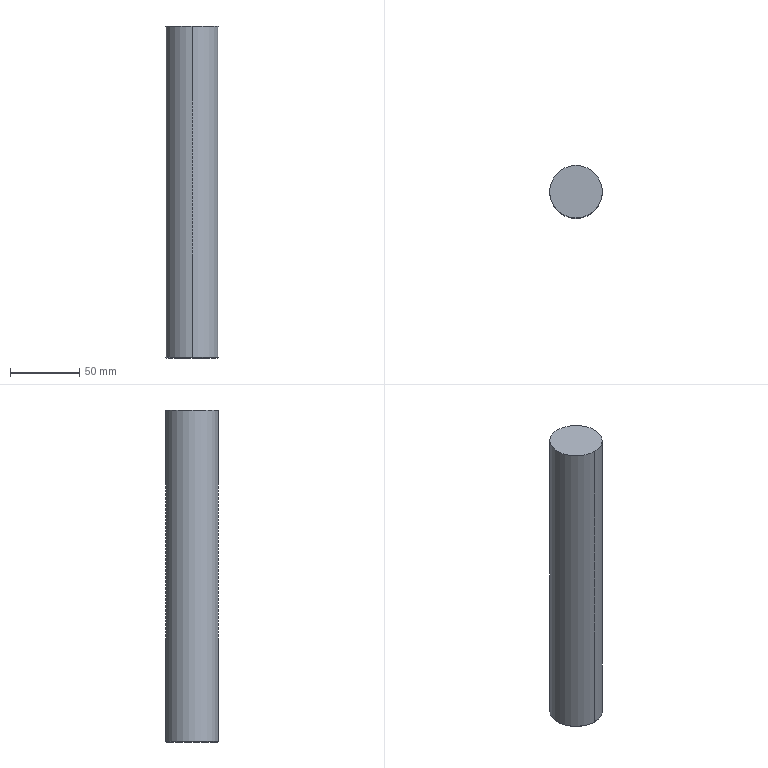Part | NX | features MYKP38-240_3 2 | 1 solid | 6 faces | box 38 x 38 x 240 mm | volume 272173 mm3 | cone 2 | plane 2 | cylinder 2 | commonest cylinder face diameters 38 x2
STEP:
#1=CARTESIAN_POINT('',(-420.023,300.595,-48.37));
#2=VERTEX_POINT('',#1);
#3=CARTESIAN_POINT('',(-420.023,300.095,-48.87));
#4=VERTEX_POINT('',#3);
#5=CARTESIAN_POINT('',(-420.023,300.095,-48.87));
#6=DIRECTION('',(0.000000003,0.7071,0.7071));
#7=VECTOR('',#6,1000.);
#8=LINE('',#5,#7);
#9=EDGE_CURVE('',#2,#4,#8,.F.);
#10=ORIENTED_EDGE('',*,*,#9,.F.);
#11=CARTESIAN_POINT('',(-420.023,262.595,-48.37));
#12=VERTEX_POINT('',#11);
#13=CARTESIAN_POINT('',(-420.023,281.595,-48.37));
#14=DIRECTION('',(0.,0.,-1.));
#15=DIRECTION('',(0.,1.,0.));
#16=AXIS2_PLACEMENT_3D('',#13,#14,#15);
#17=CIRCLE('',#16,19.);
#18=EDGE_CURVE('',#2,#12,#17,.T.);
#19=ORIENTED_EDGE('',*,*,#18,.T.);
#20=CARTESIAN_POINT('',(-420.023,263.095,-48.87));
#21=VERTEX_POINT('',#20);
#22=CARTESIAN_POINT('',(-420.023,263.095,-48.87));
#23=DIRECTION('',(-0.000000003,-0.7071,0.7071));
#24=VECTOR('',#23,1000.);
#25=LINE('',#22,#24);
#26=EDGE_CURVE('',#21,#12,#25,.T.);
#27=ORIENTED_EDGE('',*,*,#26,.F.);
#28=CARTESIAN_POINT('',(-420.023,281.595,-48.87));
#29=DIRECTION('',(0.,0.,-1.));
#30=DIRECTION('',(0.,1.,0.));
#31=AXIS2_PLACEMENT_3D('',#28,#29,#30);
#32=CIRCLE('',#31,18.5);
#33=EDGE_CURVE('',#4,#21,#32,.T.);
#34=ORIENTED_EDGE('',*,*,#33,.F.);
#35=EDGE_LOOP('',(#10,#19,#27,#34));
#36=FACE_BOUND('',#35,.T.);
#37=CARTESIAN_POINT('',(-420.023,281.595,-48.62));
#38=DIRECTION('',(0.,0.,1.));
#39=DIRECTION('',(1.,0.,0.));
#40=AXIS2_PLACEMENT_3D('',#37,#38,#39);
#41=CONICAL_SURFACE('',#40,18.75,0.7854);
#42=ADVANCED_FACE('',(#36),#41,.T.);
#43=ORIENTED_EDGE('',*,*,#26,.T.);
#44=CARTESIAN_POINT('',(-420.023,281.595,-48.37));
#45=DIRECTION('',(0.,0.,-1.));
#46=DIRECTION('',(0.,-1.,0.));
#47=AXIS2_PLACEMENT_3D('',#44,#45,#46);
#48=CIRCLE('',#47,19.);
#49=EDGE_CURVE('',#12,#2,#48,.T.);
#50=ORIENTED_EDGE('',*,*,#49,.T.);
#51=ORIENTED_EDGE('',*,*,#9,.T.);
#52=CARTESIAN_POINT('',(-420.023,281.595,-48.87));
#53=DIRECTION('',(0.,0.,-1.));
#54=DIRECTION('',(0.,-1.,0.));
#55=AXIS2_PLACEMENT_3D('',#52,#53,#54);
#56=CIRCLE('',#55,18.5);
#57=EDGE_CURVE('',#21,#4,#56,.T.);
#58=ORIENTED_EDGE('',*,*,#57,.F.);
#59=EDGE_LOOP('',(#43,#50,#51,#58));
#60=FACE_BOUND('',#59,.T.);
#61=CARTESIAN_POINT('',(-420.023,281.595,-48.62));
#62=DIRECTION('',(0.,0.,1.));
#63=DIRECTION('',(1.,0.,0.));
#64=AXIS2_PLACEMENT_3D('',#61,#62,#63);
#65=CONICAL_SURFACE('',#64,18.75,0.7854);
#66=ADVANCED_FACE('',(#60),#65,.T.);
#67=ORIENTED_EDGE('',*,*,#33,.T.);
#68=ORIENTED_EDGE('',*,*,#57,.T.);
#69=EDGE_LOOP('',(#67,#68));
#70=FACE_BOUND('',#69,.T.);
#71=CARTESIAN_POINT('',(-420.023,281.595,-48.87));
#72=DIRECTION('',(0.,0.,-1.));
#73=DIRECTION('',(0.,-1.,0.));
#74=AXIS2_PLACEMENT_3D('',#71,#72,#73);
#75=PLANE('',#74);
#76=ADVANCED_FACE('',(#70),#75,.T.);
#77=CARTESIAN_POINT('',(-420.023,300.595,138.13));
#78=VERTEX_POINT('',#77);
#79=CARTESIAN_POINT('',(-420.023,300.595,191.13));
#80=VERTEX_POINT('',#79);
#81=CARTESIAN_POINT('',(-420.023,300.595,61.63));
#82=DIRECTION('',(0.,0.000000019,1.));
#83=VECTOR('',#82,1000.);
#84=LINE('',#81,#83);
#85=EDGE_CURVE('',#78,#80,#84,.T.);
#86=ORIENTED_EDGE('',*,*,#85,.F.);
#87=CARTESIAN_POINT('',(-420.023,300.595,136.13));
#88=VERTEX_POINT('',#87);
#89=CARTESIAN_POINT('',(-420.023,300.595,61.63));
#90=DIRECTION('',(0.,0.000000019,1.));
#91=VECTOR('',#90,1000.);
#92=LINE('',#89,#91);
#93=EDGE_CURVE('',#88,#78,#92,.T.);
#94=ORIENTED_EDGE('',*,*,#93,.F.);
#95=CARTESIAN_POINT('',(-420.023,300.595,134.13));
#96=VERTEX_POINT('',#95);
#97=CARTESIAN_POINT('',(-420.023,300.595,59.63));
#98=DIRECTION('',(0.,0.000000019,1.));
#99=VECTOR('',#98,1000.);
#100=LINE('',#97,#99);
#101=EDGE_CURVE('',#96,#88,#100,.T.);
#102=ORIENTED_EDGE('',*,*,#101,.F.);
#103=CARTESIAN_POINT('',(-420.023,300.595,132.13));
#104=VERTEX_POINT('',#103);
#105=CARTESIAN_POINT('',(-420.023,300.595,57.63));
#106=DIRECTION('',(0.,0.000000019,1.));
#107=VECTOR('',#106,1000.);
#108=LINE('',#105,#107);
#109=EDGE_CURVE('',#104,#96,#108,.T.);
#110=ORIENTED_EDGE('',*,*,#109,.F.);
#111=CARTESIAN_POINT('',(-420.023,300.595,130.13));
#112=VERTEX_POINT('',#111);
#113=CARTESIAN_POINT('',(-420.023,300.595,55.63));
#114=DIRECTION('',(0.,0.000000019,1.));
#115=VECTOR('',#114,1000.);
#116=LINE('',#113,#115);
#117=EDGE_CURVE('',#112,#104,#116,.T.);
#118=ORIENTED_EDGE('',*,*,#117,.F.);
#119=CARTESIAN_POINT('',(-420.023,300.595,128.13));
#120=VERTEX_POINT('',#119);
#121=CARTESIAN_POINT('',(-420.023,300.595,53.63));
#122=DIRECTION('',(0.,0.000000019,1.));
#123=VECTOR('',#122,1000.);
#124=LINE('',#121,#123);
#125=EDGE_CURVE('',#120,#112,#124,.T.);
#126=ORIENTED_EDGE('',*,*,#125,.F.);
#127=CARTESIAN_POINT('',(-420.023,300.595,126.13));
#128=VERTEX_POINT('',#127);
#129=CARTESIAN_POINT('',(-420.023,300.595,51.63));
#130=DIRECTION('',(0.,0.000000019,1.));
#131=VECTOR('',#130,1000.);
#132=LINE('',#129,#131);
#133=EDGE_CURVE('',#128,#120,#132,.T.);
#134=ORIENTED_EDGE('',*,*,#133,.F.);
#135=CARTESIAN_POINT('',(-420.023,300.595,124.13));
#136=VERTEX_POINT('',#135);
#137=CARTESIAN_POINT('',(-420.023,300.595,49.63));
#138=DIRECTION('',(0.,0.000000019,1.));
#139=VECTOR('',#138,1000.);
#140=LINE('',#137,#139);
#141=EDGE_CURVE('',#136,#128,#140,.T.);
#142=ORIENTED_EDGE('',*,*,#141,.F.);
#143=CARTESIAN_POINT('',(-420.023,300.595,122.13));
#144=VERTEX_POINT('',#143);
#145=CARTESIAN_POINT('',(-420.023,300.595,47.63));
#146=DIRECTION('',(0.,0.000000019,1.));
#147=VECTOR('',#146,1000.);
#148=LINE('',#145,#147);
#149=EDGE_CURVE('',#144,#136,#148,.T.);
#150=ORIENTED_EDGE('',*,*,#149,.F.);
#151=CARTESIAN_POINT('',(-420.023,300.595,120.13));
#152=VERTEX_POINT('',#151);
#153=CARTESIAN_POINT('',(-420.023,300.595,45.63));
#154=DIRECTION('',(0.,0.000000019,1.));
#155=VECTOR('',#154,1000.);
#156=LINE('',#153,#155);
#157=EDGE_CURVE('',#152,#144,#156,.T.);
#158=ORIENTED_EDGE('',*,*,#157,.F.);
#159=CARTESIAN_POINT('',(-420.023,300.595,118.13));
#160=VERTEX_POINT('',#159);
#161=CARTESIAN_POINT('',(-420.023,300.595,43.63));
#162=DIRECTION('',(0.,0.000000019,1.));
#163=VECTOR('',#162,1000.);
#164=LINE('',#161,#163);
#165=EDGE_CURVE('',#160,#152,#164,.T.);
#166=ORIENTED_EDGE('',*,*,#165,.F.);
#167=CARTESIAN_POINT('',(-420.023,300.595,116.13));
#168=VERTEX_POINT('',#167);
#169=CARTESIAN_POINT('',(-420.023,300.595,41.63));
#170=DIRECTION('',(0.,0.000000019,1.));
#171=VECTOR('',#170,1000.);
#172=LINE('',#169,#171);
#173=EDGE_CURVE('',#168,#160,#172,.T.);
#174=ORIENTED_EDGE('',*,*,#173,.F.);
#175=CARTESIAN_POINT('',(-420.023,300.595,114.13));
#176=VERTEX_POINT('',#175);
#177=CARTESIAN_POINT('',(-420.023,300.595,39.63));
#178=DIRECTION('',(0.,0.000000019,1.));
#179=VECTOR('',#178,1000.);
#180=LINE('',#177,#179);
#181=EDGE_CURVE('',#176,#168,#180,.T.);
#182=ORIENTED_EDGE('',*,*,#181,.F.);
#183=CARTESIAN_POINT('',(-420.023,300.595,112.13));
#184=VERTEX_POINT('',#183);
#185=CARTESIAN_POINT('',(-420.023,300.595,37.63));
#186=DIRECTION('',(0.,0.000000019,1.));
#187=VECTOR('',#186,1000.);
#188=LINE('',#185,#187);
#189=EDGE_CURVE('',#184,#176,#188,.T.);
#190=ORIENTED_EDGE('',*,*,#189,.F.);
#191=CARTESIAN_POINT('',(-420.023,300.595,110.13));
#192=VERTEX_POINT('',#191);
#193=CARTESIAN_POINT('',(-420.023,300.595,35.63));
#194=DIRECTION('',(0.,0.000000019,1.));
#195=VECTOR('',#194,1000.);
#196=LINE('',#193,#195);
#197=EDGE_CURVE('',#192,#184,#196,.T.);
#198=ORIENTED_EDGE('',*,*,#197,.F.);
#199=CARTESIAN_POINT('',(-420.023,300.595,108.13));
#200=VERTEX_POINT('',#199);
#201=CARTESIAN_POINT('',(-420.023,300.595,33.63));
#202=DIRECTION('',(0.,0.000000019,1.));
#203=VECTOR('',#202,1000.);
#204=LINE('',#201,#203);
#205=EDGE_CURVE('',#200,#192,#204,.T.);
#206=ORIENTED_EDGE('',*,*,#205,.F.);
#207=CARTESIAN_POINT('',(-420.023,300.595,106.13));
#208=VERTEX_POINT('',#207);
#209=CARTESIAN_POINT('',(-420.023,300.595,31.63));
#210=DIRECTION('',(0.,0.000000019,1.));
#211=VECTOR('',#210,1000.);
#212=LINE('',#209,#211);
#213=EDGE_CURVE('',#208,#200,#212,.T.);
#214=ORIENTED_EDGE('',*,*,#213,.F.);
#215=CARTESIAN_POINT('',(-420.023,300.595,104.13));
#216=VERTEX_POINT('',#215);
#217=CARTESIAN_POINT('',(-420.023,300.595,29.63));
#218=DIRECTION('',(0.,0.000000019,1.));
#219=VECTOR('',#218,1000.);
#220=LINE('',#217,#219);
#221=EDGE_CURVE('',#216,#208,#220,.T.);
#222=ORIENTED_EDGE('',*,*,#221,.F.);
#223=CARTESIAN_POINT('',(-420.023,300.595,102.13));
#224=VERTEX_POINT('',#223);
#225=CARTESIAN_POINT('',(-420.023,300.595,27.63));
#226=DIRECTION('',(0.,0.000000019,1.));
#227=VECTOR('',#226,1000.);
#228=LINE('',#225,#227);
#229=EDGE_CURVE('',#224,#216,#228,.T.);
#230=ORIENTED_EDGE('',*,*,#229,.F.);
#231=CARTESIAN_POINT('',(-420.023,300.595,100.13));
#232=VERTEX_POINT('',#231);
#233=CARTESIAN_POINT('',(-420.023,300.595,25.63));
#234=DIRECTION('',(0.,0.000000019,1.));
#235=VECTOR('',#234,1000.);
#236=LINE('',#233,#235);
#237=EDGE_CURVE('',#232,#224,#236,.T.);
#238=ORIENTED_EDGE('',*,*,#237,.F.);
#239=CARTESIAN_POINT('',(-420.023,300.595,98.13));
#240=VERTEX_POINT('',#239);
#241=CARTESIAN_POINT('',(-420.023,300.595,23.63));
#242=DIRECTION('',(0.,0.000000019,1.));
#243=VECTOR('',#242,1000.);
#244=LINE('',#241,#243);
#245=EDGE_CURVE('',#240,#232,#244,.T.);
#246=ORIENTED_EDGE('',*,*,#245,.F.);
#247=CARTESIAN_POINT('',(-420.023,300.595,96.13));
#248=VERTEX_POINT('',#247);
#249=CARTESIAN_POINT('',(-420.023,300.595,21.63));
#250=DIRECTION('',(0.,0.000000019,1.));
#251=VECTOR('',#250,1000.);
#252=LINE('',#249,#251);
#253=EDGE_CURVE('',#248,#240,#252,.T.);
#254=ORIENTED_EDGE('',*,*,#253,.F.);
#255=CARTESIAN_POINT('',(-420.023,300.595,94.13));
#256=VERTEX_POINT('',#255);
#257=CARTESIAN_POINT('',(-420.023,300.595,19.63));
#258=DIRECTION('',(0.,0.000000019,1.));
#259=VECTOR('',#258,1000.);
#260=LINE('',#257,#259);
#261=EDGE_CURVE('',#256,#248,#260,.T.);
#262=ORIENTED_EDGE('',*,*,#261,.F.);
#263=CARTESIAN_POINT('',(-420.023,300.595,92.13));
#264=VERTEX_POINT('',#263);
#265=CARTESIAN_POINT('',(-420.023,300.595,17.63));
#266=DIRECTION('',(0.,0.000000019,1.));
#267=VECTOR('',#266,1000.);
#268=LINE('',#265,#267);
#269=EDGE_CURVE('',#264,#256,#268,.T.);
#270=ORIENTED_EDGE('',*,*,#269,.F.);
#271=CARTESIAN_POINT('',(-420.023,300.595,90.13));
#272=VERTEX_POINT('',#271);
#273=CARTESIAN_POINT('',(-420.023,300.595,15.63));
#274=DIRECTION('',(0.,0.000000019,1.));
#275=VECTOR('',#274,1000.);
#276=LINE('',#273,#275);
#277=EDGE_CURVE('',#272,#264,#276,.T.);
#278=ORIENTED_EDGE('',*,*,#277,.F.);
#279=CARTESIAN_POINT('',(-420.023,300.595,88.13));
#280=VERTEX_POINT('',#279);
#281=CARTESIAN_POINT('',(-420.023,300.595,13.63));
#282=DIRECTION('',(0.,0.000000019,1.));
#283=VECTOR('',#282,1000.);
#284=LINE('',#281,#283);
#285=EDGE_CURVE('',#280,#272,#284,.T.);
#286=ORIENTED_EDGE('',*,*,#285,.F.);
#287=CARTESIAN_POINT('',(-420.023,300.595,86.13));
#288=VERTEX_POINT('',#287);
#289=CARTESIAN_POINT('',(-420.023,300.595,11.63));
#290=DIRECTION('',(0.,0.000000019,1.));
#291=VECTOR('',#290,1000.);
#292=LINE('',#289,#291);
#293=EDGE_CURVE('',#288,#280,#292,.T.);
#294=ORIENTED_EDGE('',*,*,#293,.F.);
#295=CARTESIAN_POINT('',(-420.023,300.595,84.13));
#296=VERTEX_POINT('',#295);
#297=CARTESIAN_POINT('',(-420.023,300.595,9.63));
#298=DIRECTION('',(0.,0.000000019,1.));
#299=VECTOR('',#298,1000.);
#300=LINE('',#297,#299);
#301=EDGE_CURVE('',#296,#288,#300,.T.);
#302=ORIENTED_EDGE('',*,*,#301,.F.);
#303=CARTESIAN_POINT('',(-420.023,300.595,82.13));
#304=VERTEX_POINT('',#303);
#305=CARTESIAN_POINT('',(-420.023,300.595,7.63));
#306=DIRECTION('',(0.,0.000000019,1.));
#307=VECTOR('',#306,1000.);
#308=LINE('',#305,#307);
#309=EDGE_CURVE('',#304,#296,#308,.T.);
#310=ORIENTED_EDGE('',*,*,#309,.F.);
#311=CARTESIAN_POINT('',(-420.023,300.595,80.13));
#312=VERTEX_POINT('',#311);
#313=CARTESIAN_POINT('',(-420.023,300.595,5.63));
#314=DIRECTION('',(0.,0.000000019,1.));
#315=VECTOR('',#314,1000.);
#316=LINE('',#313,#315);
#317=EDGE_CURVE('',#312,#304,#316,.T.);
#318=ORIENTED_EDGE('',*,*,#317,.F.);
#319=CARTESIAN_POINT('',(-420.023,300.595,78.13));
#320=VERTEX_POINT('',#319);
#321=CARTESIAN_POINT('',(-420.023,300.595,3.63));
#322=DIRECTION('',(0.,0.000000019,1.));
#323=VECTOR('',#322,1000.);
#324=LINE('',#321,#323);
#325=EDGE_CURVE('',#320,#312,#324,.T.);
#326=ORIENTED_EDGE('',*,*,#325,.F.);
#327=CARTESIAN_POINT('',(-420.023,300.595,76.13));
#328=VERTEX_POINT('',#327);
#329=CARTESIAN_POINT('',(-420.023,300.595,1.63));
#330=DIRECTION('',(0.,0.000000019,1.));
#331=VECTOR('',#330,1000.);
#332=LINE('',#329,#331);
#333=EDGE_CURVE('',#328,#320,#332,.T.);
#334=ORIENTED_EDGE('',*,*,#333,.F.);
#335=CARTESIAN_POINT('',(-420.023,300.595,74.13));
#336=VERTEX_POINT('',#335);
#337=CARTESIAN_POINT('',(-420.023,300.595,-0.3701));
#338=DIRECTION('',(0.,0.000000019,1.));
#339=VECTOR('',#338,1000.);
#340=LINE('',#337,#339);
#341=EDGE_CURVE('',#336,#328,#340,.T.);
#342=ORIENTED_EDGE('',*,*,#341,.F.);
#343=CARTESIAN_POINT('',(-420.023,300.595,72.13));
#344=VERTEX_POINT('',#343);
#345=CARTESIAN_POINT('',(-420.023,300.595,-2.37));
#346=DIRECTION('',(0.,0.000000019,1.));
#347=VECTOR('',#346,1000.);
#348=LINE('',#345,#347);
#349=EDGE_CURVE('',#344,#336,#348,.T.);
#350=ORIENTED_EDGE('',*,*,#349,.F.);
#351=CARTESIAN_POINT('',(-420.023,300.595,70.13));
#352=VERTEX_POINT('',#351);
#353=CARTESIAN_POINT('',(-420.023,300.595,-4.37));
#354=DIRECTION('',(0.,0.000000019,1.));
#355=VECTOR('',#354,1000.);
#356=LINE('',#353,#355);
#357=EDGE_CURVE('',#352,#344,#356,.T.);
#358=ORIENTED_EDGE('',*,*,#357,.F.);
#359=CARTESIAN_POINT('',(-420.023,300.595,68.13));
#360=VERTEX_POINT('',#359);
#361=CARTESIAN_POINT('',(-420.023,300.595,-6.37));
#362=DIRECTION('',(0.,0.000000019,1.));
#363=VECTOR('',#362,1000.);
#364=LINE('',#361,#363);
#365=EDGE_CURVE('',#360,#352,#364,.T.);
#366=ORIENTED_EDGE('',*,*,#365,.F.);
#367=CARTESIAN_POINT('',(-420.023,300.595,66.13));
#368=VERTEX_POINT('',#367);
#369=CARTESIAN_POINT('',(-420.023,300.595,-8.37));
#370=DIRECTION('',(0.,0.000000019,1.));
#371=VECTOR('',#370,1000.);
#372=LINE('',#369,#371);
#373=EDGE_CURVE('',#368,#360,#372,.T.);
#374=ORIENTED_EDGE('',*,*,#373,.F.);
#375=CARTESIAN_POINT('',(-420.023,300.595,64.13));
#376=VERTEX_POINT('',#375);
#377=CARTESIAN_POINT('',(-420.023,300.595,-10.37));
#378=DIRECTION('',(0.,0.000000019,1.));
#379=VECTOR('',#378,1000.);
#380=LINE('',#377,#379);
#381=EDGE_CURVE('',#376,#368,#380,.T.);
#382=ORIENTED_EDGE('',*,*,#381,.F.);
#383=CARTESIAN_POINT('',(-420.023,300.595,62.13));
#384=VERTEX_POINT('',#383);
#385=CARTESIAN_POINT('',(-420.023,300.595,-12.37));
#386=DIRECTION('',(0.,0.000000019,1.));
#387=VECTOR('',#386,1000.);
#388=LINE('',#385,#387);
#389=EDGE_CURVE('',#384,#376,#388,.T.);
#390=ORIENTED_EDGE('',*,*,#389,.F.);
#391=CARTESIAN_POINT('',(-420.023,300.595,60.13));
#392=VERTEX_POINT('',#391);
#393=CARTESIAN_POINT('',(-420.023,300.595,-14.37));
#394=DIRECTION('',(0.,0.000000019,1.));
#395=VECTOR('',#394,1000.);
#396=LINE('',#393,#395);
#397=EDGE_CURVE('',#392,#384,#396,.T.);
#398=ORIENTED_EDGE('',*,*,#397,.F.);
#399=CARTESIAN_POINT('',(-420.023,300.595,58.13));
#400=VERTEX_POINT('',#399);
#401=CARTESIAN_POINT('',(-420.023,300.595,-16.37));
#402=DIRECTION('',(0.,0.000000019,1.));
#403=VECTOR('',#402,1000.);
#404=LINE('',#401,#403);
#405=EDGE_CURVE('',#400,#392,#404,.T.);
#406=ORIENTED_EDGE('',*,*,#405,.F.);
#407=CARTESIAN_POINT('',(-420.023,300.595,56.13));
#408=VERTEX_POINT('',#407);
#409=CARTESIAN_POINT('',(-420.023,300.595,-18.37));
#410=DIRECTION('',(0.,0.000000019,1.));
#411=VECTOR('',#410,1000.);
#412=LINE('',#409,#411);
#413=EDGE_CURVE('',#408,#400,#412,.T.);
#414=ORIENTED_EDGE('',*,*,#413,.F.);
#415=CARTESIAN_POINT('',(-420.023,300.595,54.13));
#416=VERTEX_POINT('',#415);
#417=CARTESIAN_POINT('',(-420.023,300.595,-20.37));
#418=DIRECTION('',(0.,0.000000019,1.));
#419=VECTOR('',#418,1000.);
#420=LINE('',#417,#419);
#421=EDGE_CURVE('',#416,#408,#420,.T.);
#422=ORIENTED_EDGE('',*,*,#421,.F.);
#423=CARTESIAN_POINT('',(-420.023,300.595,52.13));
#424=VERTEX_POINT('',#423);
#425=CARTESIAN_POINT('',(-420.023,300.595,-22.37));
#426=DIRECTION('',(0.,0.000000019,1.));
#427=VECTOR('',#426,1000.);
#428=LINE('',#425,#427);
#429=EDGE_CURVE('',#424,#416,#428,.T.);
#430=ORIENTED_EDGE('',*,*,#429,.F.);
#431=CARTESIAN_POINT('',(-420.023,300.595,50.13));
#432=VERTEX_POINT('',#431);
#433=CARTESIAN_POINT('',(-420.023,300.595,-24.37));
#434=DIRECTION('',(0.,0.000000019,1.));
#435=VECTOR('',#434,1000.);
#436=LINE('',#433,#435);
#437=EDGE_CURVE('',#432,#424,#436,.T.);
#438=ORIENTED_EDGE('',*,*,#437,.F.);
#439=CARTESIAN_POINT('',(-420.023,300.595,48.13));
#440=VERTEX_POINT('',#439);
#441=CARTESIAN_POINT('',(-420.023,300.595,-26.37));
#442=DIRECTION('',(0.,0.000000019,1.));
#443=VECTOR('',#442,1000.);
#444=LINE('',#441,#443);
#445=EDGE_CURVE('',#440,#432,#444,.T.);
#446=ORIENTED_EDGE('',*,*,#445,.F.);
#447=CARTESIAN_POINT('',(-420.023,300.595,46.13));
#448=VERTEX_POINT('',#447);
#449=CARTESIAN_POINT('',(-420.023,300.595,-28.37));
#450=DIRECTION('',(0.,0.000000019,1.));
#451=VECTOR('',#450,1000.);
#452=LINE('',#449,#451);
#453=EDGE_CURVE('',#448,#440,#452,.T.);
#454=ORIENTED_EDGE('',*,*,#453,.F.);
#455=CARTESIAN_POINT('',(-420.023,300.595,44.13));
#456=VERTEX_POINT('',#455);
#457=CARTESIAN_POINT('',(-420.023,300.595,-30.37));
#458=DIRECTION('',(0.,0.000000019,1.));
#459=VECTOR('',#458,1000.);
#460=LINE('',#457,#459);
#461=EDGE_CURVE('',#456,#448,#460,.T.);
#462=ORIENTED_EDGE('',*,*,#461,.F.);
#463=CARTESIAN_POINT('',(-420.023,300.595,42.13));
#464=VERTEX_POINT('',#463);
#465=CARTESIAN_POINT('',(-420.023,300.595,-32.37));
#466=DIRECTION('',(0.,0.000000019,1.));
#467=VECTOR('',#466,1000.);
#468=LINE('',#465,#467);
#469=EDGE_CURVE('',#464,#456,#468,.T.);
#470=ORIENTED_EDGE('',*,*,#469,.F.);
#471=CARTESIAN_POINT('',(-420.023,300.595,40.13));
#472=VERTEX_POINT('',#471);
#473=CARTESIAN_POINT('',(-420.023,300.595,-34.37));
#474=DIRECTION('',(0.,0.000000019,1.));
#475=VECTOR('',#474,1000.);
#476=LINE('',#473,#475);
#477=EDGE_CURVE('',#472,#464,#476,.T.);
#478=ORIENTED_EDGE('',*,*,#477,.F.);
#479=CARTESIAN_POINT('',(-420.023,300.595,38.13));
#480=VERTEX_POINT('',#479);
#481=CARTESIAN_POINT('',(-420.023,300.595,-36.37));
#482=DIRECTION('',(0.,0.000000019,1.));
#483=VECTOR('',#482,1000.);
#484=LINE('',#481,#483);
#485=EDGE_CURVE('',#480,#472,#484,.T.);
#486=ORIENTED_EDGE('',*,*,#485,.F.);
#487=CARTESIAN_POINT('',(-420.023,300.595,36.13));
#488=VERTEX_POINT('',#487);
#489=CARTESIAN_POINT('',(-420.023,300.595,-38.37));
#490=DIRECTION('',(0.,0.000000019,1.));
#491=VECTOR('',#490,1000.);
#492=LINE('',#489,#491);
#493=EDGE_CURVE('',#488,#480,#492,.T.);
#494=ORIENTED_EDGE('',*,*,#493,.F.);
#495=CARTESIAN_POINT('',(-420.023,300.595,34.13));
#496=VERTEX_POINT('',#495);
#497=CARTESIAN_POINT('',(-420.023,300.595,-40.37));
#498=DIRECTION('',(0.,0.000000019,1.));
#499=VECTOR('',#498,1000.);
#500=LINE('',#497,#499);
#501=EDGE_CURVE('',#496,#488,#500,.T.);
#502=ORIENTED_EDGE('',*,*,#501,.F.);
#503=CARTESIAN_POINT('',(-420.023,300.595,32.13));
#504=VERTEX_POINT('',#503);
#505=CARTESIAN_POINT('',(-420.023,300.595,-42.37));
#506=DIRECTION('',(0.,0.000000019,1.));
#507=VECTOR('',#506,1000.);
#508=LINE('',#505,#507);
#509=EDGE_CURVE('',#504,#496,#508,.T.);
#510=ORIENTED_EDGE('',*,*,#509,.F.);
#511=CARTESIAN_POINT('',(-420.023,300.595,30.13));
#512=VERTEX_POINT('',#511);
#513=CARTESIAN_POINT('',(-420.023,300.595,-44.37));
#514=DIRECTION('',(0.,0.000000019,1.));
#515=VECTOR('',#514,1000.);
#516=LINE('',#513,#515);
#517=EDGE_CURVE('',#512,#504,#516,.T.);
#518=ORIENTED_EDGE('',*,*,#517,.F.);
#519=CARTESIAN_POINT('',(-420.023,300.595,28.13));
#520=VERTEX_POINT('',#519);
#521=CARTESIAN_POINT('',(-420.023,300.595,-46.37));
#522=DIRECTION('',(0.,0.000000019,1.));
#523=VECTOR('',#522,1000.);
#524=LINE('',#521,#523);
#525=EDGE_CURVE('',#520,#512,#524,.T.);
#526=ORIENTED_EDGE('',*,*,#525,.F.);
#527=CARTESIAN_POINT('',(-420.023,300.595,26.13));
#528=VERTEX_POINT('',#527);
#529=CARTESIAN_POINT('',(-420.023,300.595,-48.37));
#530=DIRECTION('',(0.,0.000000019,1.));
#531=VECTOR('',#530,1000.);
#532=LINE('',#529,#531);
#533=EDGE_CURVE('',#528,#520,#532,.T.);
#534=ORIENTED_EDGE('',*,*,#533,.F.);
#535=CARTESIAN_POINT('',(-420.023,300.595,-48.37));
#536=DIRECTION('',(0.,0.000000019,1.));
#537=VECTOR('',#536,1000.);
#538=LINE('',#535,#537);
#539=EDGE_CURVE('',#2,#528,#538,.T.);
#540=ORIENTED_EDGE('',*,*,#539,.F.);
#541=ORIENTED_EDGE('',*,*,#49,.F.);
#542=CARTESIAN_POINT('',(-420.023,262.595,26.13));
#543=VERTEX_POINT('',#542);
#544=CARTESIAN_POINT('',(-420.023,262.595,-48.37));
#545=DIRECTION('',(0.,-0.000000019,1.));
#546=VECTOR('',#545,1000.);
#547=LINE('',#544,#546);
#548=EDGE_CURVE('',#543,#12,#547,.F.);
#549=ORIENTED_EDGE('',*,*,#548,.F.);
#550=CARTESIAN_POINT('',(-420.023,262.595,28.13));
#551=VERTEX_POINT('',#550);
#552=CARTESIAN_POINT('',(-420.023,262.595,-48.37));
#553=DIRECTION('',(0.,-0.000000019,1.));
#554=VECTOR('',#553,1000.);
#555=LINE('',#552,#554);
#556=EDGE_CURVE('',#551,#543,#555,.F.);
#557=ORIENTED_EDGE('',*,*,#556,.F.);
#558=CARTESIAN_POINT('',(-420.023,262.595,30.13));
#559=VERTEX_POINT('',#558);
#560=CARTESIAN_POINT('',(-420.023,262.595,-46.37));
#561=DIRECTION('',(0.,-0.000000019,1.));
#562=VECTOR('',#561,1000.);
#563=LINE('',#560,#562);
#564=EDGE_CURVE('',#559,#551,#563,.F.);
#565=ORIENTED_EDGE('',*,*,#564,.F.);
#566=CARTESIAN_POINT('',(-420.023,262.595,32.13));
#567=VERTEX_POINT('',#566);
#568=CARTESIAN_POINT('',(-420.023,262.595,-44.37));
#569=DIRECTION('',(0.,-0.000000019,1.));
#570=VECTOR('',#569,1000.);
#571=LINE('',#568,#570);
#572=EDGE_CURVE('',#567,#559,#571,.F.);
#573=ORIENTED_EDGE('',*,*,#572,.F.);
#574=CARTESIAN_POINT('',(-420.023,262.595,34.13));
#575=VERTEX_POINT('',#574);
#576=CARTESIAN_POINT('',(-420.023,262.595,-42.37));
#577=DIRECTION('',(0.,-0.000000019,1.));
#578=VECTOR('',#577,1000.);
#579=LINE('',#576,#578);
#580=EDGE_CURVE('',#575,#567,#579,.F.);
#581=ORIENTED_EDGE('',*,*,#580,.F.);
#582=CARTESIAN_POINT('',(-420.023,262.595,36.13));
#583=VERTEX_POINT('',#582);
#584=CARTESIAN_POINT('',(-420.023,262.595,-40.37));
#585=DIRECTION('',(0.,-0.000000019,1.));
#586=VECTOR('',#585,1000.);
#587=LINE('',#584,#586);
#588=EDGE_CURVE('',#583,#575,#587,.F.);
#589=ORIENTED_EDGE('',*,*,#588,.F.);
#590=CARTESIAN_POINT('',(-420.023,262.595,38.13));
#591=VERTEX_POINT('',#590);
#592=CARTESIAN_POINT('',(-420.023,262.595,-38.37));
#593=DIRECTION('',(0.,-0.000000019,1.));
#594=VECTOR('',#593,1000.);
#595=LINE('',#592,#594);
#596=EDGE_CURVE('',#591,#583,#595,.F.);
#597=ORIENTED_EDGE('',*,*,#596,.F.);
#598=CARTESIAN_POINT('',(-420.023,262.595,40.13));
#599=VERTEX_POINT('',#598);
#600=CARTESIAN_POINT('',(-420.023,262.595,-36.37));
#601=DIRECTION('',(0.,-0.000000019,1.));
#602=VECTOR('',#601,1000.);
#603=LINE('',#600,#602);
#604=EDGE_CURVE('',#599,#591,#603,.F.);
#605=ORIENTED_EDGE('',*,*,#604,.F.);
#606=CARTESIAN_POINT('',(-420.023,262.595,42.13));
#607=VERTEX_POINT('',#606);
#608=CARTESIAN_POINT('',(-420.023,262.595,-34.37));
#609=DIRECTION('',(0.,-0.000000019,1.));
#610=VECTOR('',#609,1000.);
#611=LINE('',#608,#610);
#612=EDGE_CURVE('',#607,#599,#611,.F.);
#613=ORIENTED_EDGE('',*,*,#612,.F.);
#614=CARTESIAN_POINT('',(-420.023,262.595,44.13));
#615=VERTEX_POINT('',#614);
#616=CARTESIAN_POINT('',(-420.023,262.595,-32.37));
#617=DIRECTION('',(0.,-0.000000019,1.));
#618=VECTOR('',#617,1000.);
#619=LINE('',#616,#618);
#620=EDGE_CURVE('',#615,#607,#619,.F.);
#621=ORIENTED_EDGE('',*,*,#620,.F.);
#622=CARTESIAN_POINT('',(-420.023,262.595,46.13));
#623=VERTEX_POINT('',#622);
#624=CARTESIAN_POINT('',(-420.023,262.595,-30.37));
#625=DIRECTION('',(0.,-0.000000019,1.));
#626=VECTOR('',#625,1000.);
#627=LINE('',#624,#626);
#628=EDGE_CURVE('',#623,#615,#627,.F.);
#629=ORIENTED_EDGE('',*,*,#628,.F.);
#630=CARTESIAN_POINT('',(-420.023,262.595,48.13));
#631=VERTEX_POINT('',#630);
#632=CARTESIAN_POINT('',(-420.023,262.595,-28.37));
#633=DIRECTION('',(0.,-0.000000019,1.));
#634=VECTOR('',#633,1000.);
#635=LINE('',#632,#634);
#636=EDGE_CURVE('',#631,#623,#635,.F.);
#637=ORIENTED_EDGE('',*,*,#636,.F.);
#638=CARTESIAN_POINT('',(-420.023,262.595,50.13));
#639=VERTEX_POINT('',#638);
#640=CARTESIAN_POINT('',(-420.023,262.595,-26.37));
#641=DIRECTION('',(0.,-0.000000019,1.));
#642=VECTOR('',#641,1000.);
#643=LINE('',#640,#642);
#644=EDGE_CURVE('',#639,#631,#643,.F.);
#645=ORIENTED_EDGE('',*,*,#644,.F.);
#646=CARTESIAN_POINT('',(-420.023,262.595,52.13));
#647=VERTEX_POINT('',#646);
#648=CARTESIAN_POINT('',(-420.023,262.595,-24.37));
#649=DIRECTION('',(0.,-0.000000019,1.));
#650=VECTOR('',#649,1000.);
#651=LINE('',#648,#650);
#652=EDGE_CURVE('',#647,#639,#651,.F.);
#653=ORIENTED_EDGE('',*,*,#652,.F.);
#654=CARTESIAN_POINT('',(-420.023,262.595,54.13));
#655=VERTEX_POINT('',#654);
#656=CARTESIAN_POINT('',(-420.023,262.595,-22.37));
#657=DIRECTION('',(0.,-0.000000019,1.));
#658=VECTOR('',#657,1000.);
#659=LINE('',#656,#658);
#660=EDGE_CURVE('',#655,#647,#659,.F.);
#661=ORIENTED_EDGE('',*,*,#660,.F.);
#662=CARTESIAN_POINT('',(-420.023,262.595,56.13));
#663=VERTEX_POINT('',#662);
#664=CARTESIAN_POINT('',(-420.023,262.595,-20.37));
#665=DIRECTION('',(0.,-0.000000019,1.));
#666=VECTOR('',#665,1000.);
#667=LINE('',#664,#666);
#668=EDGE_CURVE('',#663,#655,#667,.F.);
#669=ORIENTED_EDGE('',*,*,#668,.F.);
#670=CARTESIAN_POINT('',(-420.023,262.595,58.13));
#671=VERTEX_POINT('',#670);
#672=CARTESIAN_POINT('',(-420.023,262.595,-18.37));
#673=DIRECTION('',(0.,-0.000000019,1.));
#674=VECTOR('',#673,1000.);
#675=LINE('',#672,#674);
#676=EDGE_CURVE('',#671,#663,#675,.F.);
#677=ORIENTED_EDGE('',*,*,#676,.F.);
#678=CARTESIAN_POINT('',(-420.023,262.595,60.13));
#679=VERTEX_POINT('',#678);
#680=CARTESIAN_POINT('',(-420.023,262.595,-16.37));
#681=DIRECTION('',(0.,-0.000000019,1.));
#682=VECTOR('',#681,1000.);
#683=LINE('',#680,#682);
#684=EDGE_CURVE('',#679,#671,#683,.F.);
#685=ORIENTED_EDGE('',*,*,#684,.F.);
#686=CARTESIAN_POINT('',(-420.023,262.595,62.13));
#687=VERTEX_POINT('',#686);
#688=CARTESIAN_POINT('',(-420.023,262.595,-14.37));
#689=DIRECTION('',(0.,-0.000000019,1.));
#690=VECTOR('',#689,1000.);
#691=LINE('',#688,#690);
#692=EDGE_CURVE('',#687,#679,#691,.F.);
#693=ORIENTED_EDGE('',*,*,#692,.F.);
#694=CARTESIAN_POINT('',(-420.023,262.595,64.13));
#695=VERTEX_POINT('',#694);
#696=CARTESIAN_POINT('',(-420.023,262.595,-12.37));
#697=DIRECTION('',(0.,-0.000000019,1.));
#698=VECTOR('',#697,1000.);
#699=LINE('',#696,#698);
#700=EDGE_CURVE('',#695,#687,#699,.F.);
#701=ORIENTED_EDGE('',*,*,#700,.F.);
#702=CARTESIAN_POINT('',(-420.023,262.595,66.13));
#703=VERTEX_POINT('',#702);
#704=CARTESIAN_POINT('',(-420.023,262.595,-10.37));
#705=DIRECTION('',(0.,-0.000000019,1.));
#706=VECTOR('',#705,1000.);
#707=LINE('',#704,#706);
#708=EDGE_CURVE('',#703,#695,#707,.F.);
#709=ORIENTED_EDGE('',*,*,#708,.F.);
#710=CARTESIAN_POINT('',(-420.023,262.595,68.13));
#711=VERTEX_POINT('',#710);
#712=CARTESIAN_POINT('',(-420.023,262.595,-8.37));
#713=DIRECTION('',(0.,-0.000000019,1.));
#714=VECTOR('',#713,1000.);
#715=LINE('',#712,#714);
#716=EDGE_CURVE('',#711,#703,#715,.F.);
#717=ORIENTED_EDGE('',*,*,#716,.F.);
#718=CARTESIAN_POINT('',(-420.023,262.595,70.13));
#719=VERTEX_POINT('',#718);
#720=CARTESIAN_POINT('',(-420.023,262.595,-6.37));
#721=DIRECTION('',(0.,-0.000000019,1.));
#722=VECTOR('',#721,1000.);
#723=LINE('',#720,#722);
#724=EDGE_CURVE('',#719,#711,#723,.F.);
#725=ORIENTED_EDGE('',*,*,#724,.F.);
#726=CARTESIAN_POINT('',(-420.023,262.595,72.13));
#727=VERTEX_POINT('',#726);
#728=CARTESIAN_POINT('',(-420.023,262.595,-4.37));
#729=DIRECTION('',(0.,-0.000000019,1.));
#730=VECTOR('',#729,1000.);
#731=LINE('',#728,#730);
#732=EDGE_CURVE('',#727,#719,#731,.F.);
#733=ORIENTED_EDGE('',*,*,#732,.F.);
#734=CARTESIAN_POINT('',(-420.023,262.595,74.13));
#735=VERTEX_POINT('',#734);
#736=CARTESIAN_POINT('',(-420.023,262.595,-2.37));
#737=DIRECTION('',(0.,-0.000000019,1.));
#738=VECTOR('',#737,1000.);
#739=LINE('',#736,#738);
#740=EDGE_CURVE('',#735,#727,#739,.F.);
#741=ORIENTED_EDGE('',*,*,#740,.F.);
#742=CARTESIAN_POINT('',(-420.023,262.595,76.13));
#743=VERTEX_POINT('',#742);
#744=CARTESIAN_POINT('',(-420.023,262.595,-0.3701));
#745=DIRECTION('',(0.,-0.000000019,1.));
#746=VECTOR('',#745,1000.);
#747=LINE('',#744,#746);
#748=EDGE_CURVE('',#743,#735,#747,.F.);
#749=ORIENTED_EDGE('',*,*,#748,.F.);
#750=CARTESIAN_POINT('',(-420.023,262.595,78.13));
#751=VERTEX_POINT('',#750);
#752=CARTESIAN_POINT('',(-420.023,262.595,1.63));
#753=DIRECTION('',(0.,-0.000000019,1.));
#754=VECTOR('',#753,1000.);
#755=LINE('',#752,#754);
#756=EDGE_CURVE('',#751,#743,#755,.F.);
#757=ORIENTED_EDGE('',*,*,#756,.F.);
#758=CARTESIAN_POINT('',(-420.023,262.595,80.13));
#759=VERTEX_POINT('',#758);
#760=CARTESIAN_POINT('',(-420.023,262.595,3.63));
#761=DIRECTION('',(0.,-0.000000019,1.));
#762=VECTOR('',#761,1000.);
#763=LINE('',#760,#762);
#764=EDGE_CURVE('',#759,#751,#763,.F.);
#765=ORIENTED_EDGE('',*,*,#764,.F.);
#766=CARTESIAN_POINT('',(-420.023,262.595,82.13));
#767=VERTEX_POINT('',#766);
#768=CARTESIAN_POINT('',(-420.023,262.595,5.63));
#769=DIRECTION('',(0.,-0.000000019,1.));
#770=VECTOR('',#769,1000.);
#771=LINE('',#768,#770);
#772=EDGE_CURVE('',#767,#759,#771,.F.);
#773=ORIENTED_EDGE('',*,*,#772,.F.);
#774=CARTESIAN_POINT('',(-420.023,262.595,84.13));
#775=VERTEX_POINT('',#774);
#776=CARTESIAN_POINT('',(-420.023,262.595,7.63));
#777=DIRECTION('',(0.,-0.000000019,1.));
#778=VECTOR('',#777,1000.);
#779=LINE('',#776,#778);
#780=EDGE_CURVE('',#775,#767,#779,.F.);
#781=ORIENTED_EDGE('',*,*,#780,.F.);
#782=CARTESIAN_POINT('',(-420.023,262.595,86.13));
#783=VERTEX_POINT('',#782);
#784=CARTESIAN_POINT('',(-420.023,262.595,9.63));
#785=DIRECTION('',(0.,-0.000000019,1.));
#786=VECTOR('',#785,1000.);
#787=LINE('',#784,#786);
#788=EDGE_CURVE('',#783,#775,#787,.F.);
#789=ORIENTED_EDGE('',*,*,#788,.F.);
#790=CARTESIAN_POINT('',(-420.023,262.595,88.13));
#791=VERTEX_POINT('',#790);
#792=CARTESIAN_POINT('',(-420.023,262.595,11.63));
#793=DIRECTION('',(0.,-0.000000019,1.));
#794=VECTOR('',#793,1000.);
#795=LINE('',#792,#794);
#796=EDGE_CURVE('',#791,#783,#795,.F.);
#797=ORIENTED_EDGE('',*,*,#796,.F.);
#798=CARTESIAN_POINT('',(-420.023,262.595,90.13));
#799=VERTEX_POINT('',#798);
#800=CARTESIAN_POINT('',(-420.023,262.595,13.63));
#801=DIRECTION('',(0.,-0.000000019,1.));
#802=VECTOR('',#801,1000.);
#803=LINE('',#800,#802);
#804=EDGE_CURVE('',#799,#791,#803,.F.);
#805=ORIENTED_EDGE('',*,*,#804,.F.);
#806=CARTESIAN_POINT('',(-420.023,262.595,92.13));
#807=VERTEX_POINT('',#806);
#808=CARTESIAN_POINT('',(-420.023,262.595,15.63));
#809=DIRECTION('',(0.,-0.000000019,1.));
#810=VECTOR('',#809,1000.);
#811=LINE('',#808,#810);
#812=EDGE_CURVE('',#807,#799,#811,.F.);
#813=ORIENTED_EDGE('',*,*,#812,.F.);
#814=CARTESIAN_POINT('',(-420.023,262.595,94.13));
#815=VERTEX_POINT('',#814);
#816=CARTESIAN_POINT('',(-420.023,262.595,17.63));
#817=DIRECTION('',(0.,-0.000000019,1.));
#818=VECTOR('',#817,1000.);
#819=LINE('',#816,#818);
#820=EDGE_CURVE('',#815,#807,#819,.F.);
#821=ORIENTED_EDGE('',*,*,#820,.F.);
#822=CARTESIAN_POINT('',(-420.023,262.595,96.13));
#823=VERTEX_POINT('',#822);
#824=CARTESIAN_POINT('',(-420.023,262.595,19.63));
#825=DIRECTION('',(0.,-0.000000019,1.));
#826=VECTOR('',#825,1000.);
#827=LINE('',#824,#826);
#828=EDGE_CURVE('',#823,#815,#827,.F.);
#829=ORIENTED_EDGE('',*,*,#828,.F.);
#830=CARTESIAN_POINT('',(-420.023,262.595,98.13));
#831=VERTEX_POINT('',#830);
#832=CARTESIAN_POINT('',(-420.023,262.595,21.63));
#833=DIRECTION('',(0.,-0.000000019,1.));
#834=VECTOR('',#833,1000.);
#835=LINE('',#832,#834);
#836=EDGE_CURVE('',#831,#823,#835,.F.);
#837=ORIENTED_EDGE('',*,*,#836,.F.);
#838=CARTESIAN_POINT('',(-420.023,262.595,100.13));
#839=VERTEX_POINT('',#838);
#840=CARTESIAN_POINT('',(-420.023,262.595,23.63));
#841=DIRECTION('',(0.,-0.000000019,1.));
#842=VECTOR('',#841,1000.);
#843=LINE('',#840,#842);
#844=EDGE_CURVE('',#839,#831,#843,.F.);
#845=ORIENTED_EDGE('',*,*,#844,.F.);
#846=CARTESIAN_POINT('',(-420.023,262.595,102.13));
#847=VERTEX_POINT('',#846);
#848=CARTESIAN_POINT('',(-420.023,262.595,25.63));
#849=DIRECTION('',(0.,-0.000000019,1.));
#850=VECTOR('',#849,1000.);
#851=LINE('',#848,#850);
#852=EDGE_CURVE('',#847,#839,#851,.F.);
#853=ORIENTED_EDGE('',*,*,#852,.F.);
#854=CARTESIAN_POINT('',(-420.023,262.595,104.13));
#855=VERTEX_POINT('',#854);
#856=CARTESIAN_POINT('',(-420.023,262.595,27.63));
#857=DIRECTION('',(0.,-0.000000019,1.));
#858=VECTOR('',#857,1000.);
#859=LINE('',#856,#858);
#860=EDGE_CURVE('',#855,#847,#859,.F.);
#861=ORIENTED_EDGE('',*,*,#860,.F.);
#862=CARTESIAN_POINT('',(-420.023,262.595,106.13));
#863=VERTEX_POINT('',#862);
#864=CARTESIAN_POINT('',(-420.023,262.595,29.63));
#865=DIRECTION('',(0.,-0.000000019,1.));
#866=VECTOR('',#865,1000.);
#867=LINE('',#864,#866);
#868=EDGE_CURVE('',#863,#855,#867,.F.);
#869=ORIENTED_EDGE('',*,*,#868,.F.);
#870=CARTESIAN_POINT('',(-420.023,262.595,108.13));
#871=VERTEX_POINT('',#870);
#872=CARTESIAN_POINT('',(-420.023,262.595,31.63));
#873=DIRECTION('',(0.,-0.000000019,1.));
#874=VECTOR('',#873,1000.);
#875=LINE('',#872,#874);
#876=EDGE_CURVE('',#871,#863,#875,.F.);
#877=ORIENTED_EDGE('',*,*,#876,.F.);
#878=CARTESIAN_POINT('',(-420.023,262.595,110.13));
#879=VERTEX_POINT('',#878);
#880=CARTESIAN_POINT('',(-420.023,262.595,33.63));
#881=DIRECTION('',(0.,-0.000000019,1.));
#882=VECTOR('',#881,1000.);
#883=LINE('',#880,#882);
#884=EDGE_CURVE('',#879,#871,#883,.F.);
#885=ORIENTED_EDGE('',*,*,#884,.F.);
#886=CARTESIAN_POINT('',(-420.023,262.595,112.13));
#887=VERTEX_POINT('',#886);
#888=CARTESIAN_POINT('',(-420.023,262.595,35.63));
#889=DIRECTION('',(0.,-0.000000019,1.));
#890=VECTOR('',#889,1000.);
#891=LINE('',#888,#890);
#892=EDGE_CURVE('',#887,#879,#891,.F.);
#893=ORIENTED_EDGE('',*,*,#892,.F.);
#894=CARTESIAN_POINT('',(-420.023,262.595,114.13));
#895=VERTEX_POINT('',#894);
#896=CARTESIAN_POINT('',(-420.023,262.595,37.63));
#897=DIRECTION('',(0.,-0.000000019,1.));
#898=VECTOR('',#897,1000.);
#899=LINE('',#896,#898);
#900=EDGE_CURVE('',#895,#887,#899,.F.);
#901=ORIENTED_EDGE('',*,*,#900,.F.);
#902=CARTESIAN_POINT('',(-420.023,262.595,116.13));
#903=VERTEX_POINT('',#902);
#904=CARTESIAN_POINT('',(-420.023,262.595,39.63));
#905=DIRECTION('',(0.,-0.000000019,1.));
#906=VECTOR('',#905,1000.);
#907=LINE('',#904,#906);
#908=EDGE_CURVE('',#903,#895,#907,.F.);
#909=ORIENTED_EDGE('',*,*,#908,.F.);
#910=CARTESIAN_POINT('',(-420.023,262.595,118.13));
#911=VERTEX_POINT('',#910);
#912=CARTESIAN_POINT('',(-420.023,262.595,41.63));
#913=DIRECTION('',(0.,-0.000000019,1.));
#914=VECTOR('',#913,1000.);
#915=LINE('',#912,#914);
#916=EDGE_CURVE('',#911,#903,#915,.F.);
#917=ORIENTED_EDGE('',*,*,#916,.F.);
#918=CARTESIAN_POINT('',(-420.023,262.595,120.13));
#919=VERTEX_POINT('',#918);
#920=CARTESIAN_POINT('',(-420.023,262.595,43.63));
#921=DIRECTION('',(0.,-0.000000019,1.));
#922=VECTOR('',#921,1000.);
#923=LINE('',#920,#922);
#924=EDGE_CURVE('',#919,#911,#923,.F.);
#925=ORIENTED_EDGE('',*,*,#924,.F.);
#926=CARTESIAN_POINT('',(-420.023,262.595,122.13));
#927=VERTEX_POINT('',#926);
#928=CARTESIAN_POINT('',(-420.023,262.595,45.63));
#929=DIRECTION('',(0.,-0.000000019,1.));
#930=VECTOR('',#929,1000.);
#931=LINE('',#928,#930);
#932=EDGE_CURVE('',#927,#919,#931,.F.);
#933=ORIENTED_EDGE('',*,*,#932,.F.);
#934=CARTESIAN_POINT('',(-420.023,262.595,124.13));
#935=VERTEX_POINT('',#934);
#936=CARTESIAN_POINT('',(-420.023,262.595,47.63));
#937=DIRECTION('',(0.,-0.000000019,1.));
#938=VECTOR('',#937,1000.);
#939=LINE('',#936,#938);
#940=EDGE_CURVE('',#935,#927,#939,.F.);
#941=ORIENTED_EDGE('',*,*,#940,.F.);
#942=CARTESIAN_POINT('',(-420.023,262.595,126.13));
#943=VERTEX_POINT('',#942);
#944=CARTESIAN_POINT('',(-420.023,262.595,49.63));
#945=DIRECTION('',(0.,-0.000000019,1.));
#946=VECTOR('',#945,1000.);
#947=LINE('',#944,#946);
#948=EDGE_CURVE('',#943,#935,#947,.F.);
#949=ORIENTED_EDGE('',*,*,#948,.F.);
#950=CARTESIAN_POINT('',(-420.023,262.595,128.13));
#951=VERTEX_POINT('',#950);
#952=CARTESIAN_POINT('',(-420.023,262.595,51.63));
#953=DIRECTION('',(0.,-0.000000019,1.));
#954=VECTOR('',#953,1000.);
#955=LINE('',#952,#954);
#956=EDGE_CURVE('',#951,#943,#955,.F.);
#957=ORIENTED_EDGE('',*,*,#956,.F.);
#958=CARTESIAN_POINT('',(-420.023,262.595,130.13));
#959=VERTEX_POINT('',#958);
#960=CARTESIAN_POINT('',(-420.023,262.595,53.63));
#961=DIRECTION('',(0.,-0.000000019,1.));
#962=VECTOR('',#961,1000.);
#963=LINE('',#960,#962);
#964=EDGE_CURVE('',#959,#951,#963,.F.);
#965=ORIENTED_EDGE('',*,*,#964,.F.);
#966=CARTESIAN_POINT('',(-420.023,262.595,132.13));
#967=VERTEX_POINT('',#966);
#968=CARTESIAN_POINT('',(-420.023,262.595,55.63));
#969=DIRECTION('',(0.,-0.000000019,1.));
#970=VECTOR('',#969,1000.);
#971=LINE('',#968,#970);
#972=EDGE_CURVE('',#967,#959,#971,.F.);
#973=ORIENTED_EDGE('',*,*,#972,.F.);
#974=CARTESIAN_POINT('',(-420.023,262.595,134.13));
#975=VERTEX_POINT('',#974);
#976=CARTESIAN_POINT('',(-420.023,262.595,57.63));
#977=DIRECTION('',(0.,-0.000000019,1.));
#978=VECTOR('',#977,1000.);
#979=LINE('',#976,#978);
#980=EDGE_CURVE('',#975,#967,#979,.F.);
#981=ORIENTED_EDGE('',*,*,#980,.F.);
#982=CARTESIAN_POINT('',(-420.023,262.595,136.13));
#983=VERTEX_POINT('',#982);
#984=CARTESIAN_POINT('',(-420.023,262.595,59.63));
#985=DIRECTION('',(0.,-0.000000019,1.));
#986=VECTOR('',#985,1000.);
#987=LINE('',#984,#986);
#988=EDGE_CURVE('',#983,#975,#987,.F.);
#989=ORIENTED_EDGE('',*,*,#988,.F.);
#990=CARTESIAN_POINT('',(-420.023,262.595,138.13));
#991=VERTEX_POINT('',#990);
#992=CARTESIAN_POINT('',(-420.023,262.595,61.63));
#993=DIRECTION('',(0.,-0.000000019,1.));
#994=VECTOR('',#993,1000.);
#995=LINE('',#992,#994);
#996=EDGE_CURVE('',#991,#983,#995,.F.);
#997=ORIENTED_EDGE('',*,*,#996,.F.);
#998=CARTESIAN_POINT('',(-420.023,262.595,191.13));
#999=VERTEX_POINT('',#998);
#1000=CARTESIAN_POINT('',(-420.023,262.595,61.63));
#1001=DIRECTION('',(0.,-0.000000019,1.));
#1002=VECTOR('',#1001,1000.);
#1003=LINE('',#1000,#1002);
#1004=EDGE_CURVE('',#999,#991,#1003,.F.);
#1005=ORIENTED_EDGE('',*,*,#1004,.F.);
#1006=CARTESIAN_POINT('',(-420.023,281.595,191.13));
#1007=DIRECTION('',(0.,0.,1.));
#1008=DIRECTION('',(0.,1.,0.));
#1009=AXIS2_PLACEMENT_3D('',#1006,#1007,#1008);
#1010=CIRCLE('',#1009,19.);
#1011=EDGE_CURVE('',#80,#999,#1010,.T.);
#1012=ORIENTED_EDGE('',*,*,#1011,.F.);
#1013=EDGE_LOOP('',(#86,#94,#102,#110,#118,#126,#134,#142,#150,#158,#166,#174,#182,#190,#198,#206,#214,#222,#230,#238,#246,#254,#262,#270,#278,#286,#294,#302,#310,#318,#326,#334,#342,#350,#358,#366,#374,#382,#390,#398,#406,#414,#422,#430,#438,#446,#454,#462,#470,#478,#486,#494,#502,#510,#518,#526,#534,#540,#541,#549,#557,#565,#573,#581,#589,#597,#605,#613,#621,#629,#637,#645,#653,#661,#669,#677,#685,#693,#701,#709,#717,#725,#733,#741,#749,#757,#765,#773,#781,#789,#797,#805,#813,#821,#829,#837,#845,#853,#861,#869,#877,#885,#893,#901,#909,#917,#925,#933,#941,#949,#957,#965,#973,#981,#989,#997,#1005,#1012));
#1014=FACE_BOUND('',#1013,.T.);
#1015=CARTESIAN_POINT('',(-420.023,281.595,61.13));
#1016=DIRECTION('',(0.,0.,-1.));
#1017=DIRECTION('',(0.,1.,0.));
#1018=AXIS2_PLACEMENT_3D('',#1015,#1016,#1017);
#1019=CYLINDRICAL_SURFACE('',#1018,19.);
#1020=ADVANCED_FACE('',(#1014),#1019,.T.);
#1021=ORIENTED_EDGE('',*,*,#1011,.T.);
#1022=CARTESIAN_POINT('',(-420.023,281.595,191.13));
#1023=DIRECTION('',(0.,0.,1.));
#1024=DIRECTION('',(0.,-1.,0.));
#1025=AXIS2_PLACEMENT_3D('',#1022,#1023,#1024);
#1026=CIRCLE('',#1025,19.);
#1027=EDGE_CURVE('',#999,#80,#1026,.T.);
#1028=ORIENTED_EDGE('',*,*,#1027,.T.);
#1029=EDGE_LOOP('',(#1021,#1028));
#1030=FACE_BOUND('',#1029,.T.);
#1031=CARTESIAN_POINT('',(-382.523,219.595,191.13));
#1032=DIRECTION('',(0.,0.,1.));
#1033=DIRECTION('',(1.,0.,0.));
#1034=AXIS2_PLACEMENT_3D('',#1031,#1032,#1033);
#1035=PLANE('',#1034);
#1036=ADVANCED_FACE('',(#1030),#1035,.T.);
#1037=ORIENTED_EDGE('',*,*,#1004,.T.);
#1038=ORIENTED_EDGE('',*,*,#996,.T.);
#1039=ORIENTED_EDGE('',*,*,#988,.T.);
#1040=ORIENTED_EDGE('',*,*,#980,.T.);
#1041=ORIENTED_EDGE('',*,*,#972,.T.);
#1042=ORIENTED_EDGE('',*,*,#964,.T.);
#1043=ORIENTED_EDGE('',*,*,#956,.T.);
#1044=ORIENTED_EDGE('',*,*,#948,.T.);
#1045=ORIENTED_EDGE('',*,*,#940,.T.);
#1046=ORIENTED_EDGE('',*,*,#932,.T.);
#1047=ORIENTED_EDGE('',*,*,#924,.T.);
#1048=ORIENTED_EDGE('',*,*,#916,.T.);
#1049=ORIENTED_EDGE('',*,*,#908,.T.);
#1050=ORIENTED_EDGE('',*,*,#900,.T.);
#1051=ORIENTED_EDGE('',*,*,#892,.T.);
#1052=ORIENTED_EDGE('',*,*,#884,.T.);
#1053=ORIENTED_EDGE('',*,*,#876,.T.);
#1054=ORIENTED_EDGE('',*,*,#868,.T.);
#1055=ORIENTED_EDGE('',*,*,#860,.T.);
#1056=ORIENTED_EDGE('',*,*,#852,.T.);
#1057=ORIENTED_EDGE('',*,*,#844,.T.);
#1058=ORIENTED_EDGE('',*,*,#836,.T.);
#1059=ORIENTED_EDGE('',*,*,#828,.T.);
#1060=ORIENTED_EDGE('',*,*,#820,.T.);
#1061=ORIENTED_EDGE('',*,*,#812,.T.);
#1062=ORIENTED_EDGE('',*,*,#804,.T.);
#1063=ORIENTED_EDGE('',*,*,#796,.T.);
#1064=ORIENTED_EDGE('',*,*,#788,.T.);
#1065=ORIENTED_EDGE('',*,*,#780,.T.);
#1066=ORIENTED_EDGE('',*,*,#772,.T.);
#1067=ORIENTED_EDGE('',*,*,#764,.T.);
#1068=ORIENTED_EDGE('',*,*,#756,.T.);
#1069=ORIENTED_EDGE('',*,*,#748,.T.);
#1070=ORIENTED_EDGE('',*,*,#740,.T.);
#1071=ORIENTED_EDGE('',*,*,#732,.T.);
#1072=ORIENTED_EDGE('',*,*,#724,.T.);
#1073=ORIENTED_EDGE('',*,*,#716,.T.);
#1074=ORIENTED_EDGE('',*,*,#708,.T.);
#1075=ORIENTED_EDGE('',*,*,#700,.T.);
#1076=ORIENTED_EDGE('',*,*,#692,.T.);
#1077=ORIENTED_EDGE('',*,*,#684,.T.);
#1078=ORIENTED_EDGE('',*,*,#676,.T.);
#1079=ORIENTED_EDGE('',*,*,#668,.T.);
#1080=ORIENTED_EDGE('',*,*,#660,.T.);
#1081=ORIENTED_EDGE('',*,*,#652,.T.);
#1082=ORIENTED_EDGE('',*,*,#644,.T.);
#1083=ORIENTED_EDGE('',*,*,#636,.T.);
#1084=ORIENTED_EDGE('',*,*,#628,.T.);
#1085=ORIENTED_EDGE('',*,*,#620,.T.);
#1086=ORIENTED_EDGE('',*,*,#612,.T.);
#1087=ORIENTED_EDGE('',*,*,#604,.T.);
#1088=ORIENTED_EDGE('',*,*,#596,.T.);
#1089=ORIENTED_EDGE('',*,*,#588,.T.);
#1090=ORIENTED_EDGE('',*,*,#580,.T.);
#1091=ORIENTED_EDGE('',*,*,#572,.T.);
#1092=ORIENTED_EDGE('',*,*,#564,.T.);
#1093=ORIENTED_EDGE('',*,*,#556,.T.);
#1094=ORIENTED_EDGE('',*,*,#548,.T.);
#1095=ORIENTED_EDGE('',*,*,#18,.F.);
#1096=ORIENTED_EDGE('',*,*,#539,.T.);
#1097=ORIENTED_EDGE('',*,*,#533,.T.);
#1098=ORIENTED_EDGE('',*,*,#525,.T.);
#1099=ORIENTED_EDGE('',*,*,#517,.T.);
#1100=ORIENTED_EDGE('',*,*,#509,.T.);
#1101=ORIENTED_EDGE('',*,*,#501,.T.);
#1102=ORIENTED_EDGE('',*,*,#493,.T.);
#1103=ORIENTED_EDGE('',*,*,#485,.T.);
#1104=ORIENTED_EDGE('',*,*,#477,.T.);
#1105=ORIENTED_EDGE('',*,*,#469,.T.);
#1106=ORIENTED_EDGE('',*,*,#461,.T.);
#1107=ORIENTED_EDGE('',*,*,#453,.T.);
#1108=ORIENTED_EDGE('',*,*,#445,.T.);
#1109=ORIENTED_EDGE('',*,*,#437,.T.);
#1110=ORIENTED_EDGE('',*,*,#429,.T.);
#1111=ORIENTED_EDGE('',*,*,#421,.T.);
#1112=ORIENTED_EDGE('',*,*,#413,.T.);
#1113=ORIENTED_EDGE('',*,*,#405,.T.);
#1114=ORIENTED_EDGE('',*,*,#397,.T.);
#1115=ORIENTED_EDGE('',*,*,#389,.T.);
#1116=ORIENTED_EDGE('',*,*,#381,.T.);
#1117=ORIENTED_EDGE('',*,*,#373,.T.);
#1118=ORIENTED_EDGE('',*,*,#365,.T.);
#1119=ORIENTED_EDGE('',*,*,#357,.T.);
#1120=ORIENTED_EDGE('',*,*,#349,.T.);
#1121=ORIENTED_EDGE('',*,*,#341,.T.);
#1122=ORIENTED_EDGE('',*,*,#333,.T.);
#1123=ORIENTED_EDGE('',*,*,#325,.T.);
#1124=ORIENTED_EDGE('',*,*,#317,.T.);
#1125=ORIENTED_EDGE('',*,*,#309,.T.);
#1126=ORIENTED_EDGE('',*,*,#301,.T.);
#1127=ORIENTED_EDGE('',*,*,#293,.T.);
#1128=ORIENTED_EDGE('',*,*,#285,.T.);
#1129=ORIENTED_EDGE('',*,*,#277,.T.);
#1130=ORIENTED_EDGE('',*,*,#269,.T.);
#1131=ORIENTED_EDGE('',*,*,#261,.T.);
#1132=ORIENTED_EDGE('',*,*,#253,.T.);
#1133=ORIENTED_EDGE('',*,*,#245,.T.);
#1134=ORIENTED_EDGE('',*,*,#237,.T.);
#1135=ORIENTED_EDGE('',*,*,#229,.T.);
#1136=ORIENTED_EDGE('',*,*,#221,.T.);
#1137=ORIENTED_EDGE('',*,*,#213,.T.);
#1138=ORIENTED_EDGE('',*,*,#205,.T.);
#1139=ORIENTED_EDGE('',*,*,#197,.T.);
#1140=ORIENTED_EDGE('',*,*,#189,.T.);
#1141=ORIENTED_EDGE('',*,*,#181,.T.);
#1142=ORIENTED_EDGE('',*,*,#173,.T.);
#1143=ORIENTED_EDGE('',*,*,#165,.T.);
#1144=ORIENTED_EDGE('',*,*,#157,.T.);
#1145=ORIENTED_EDGE('',*,*,#149,.T.);
#1146=ORIENTED_EDGE('',*,*,#141,.T.);
#1147=ORIENTED_EDGE('',*,*,#133,.T.);
#1148=ORIENTED_EDGE('',*,*,#125,.T.);
#1149=ORIENTED_EDGE('',*,*,#117,.T.);
#1150=ORIENTED_EDGE('',*,*,#109,.T.);
#1151=ORIENTED_EDGE('',*,*,#101,.T.);
#1152=ORIENTED_EDGE('',*,*,#93,.T.);
#1153=ORIENTED_EDGE('',*,*,#85,.T.);
#1154=ORIENTED_EDGE('',*,*,#1027,.F.);
#1155=EDGE_LOOP('',(#1037,#1038,#1039,#1040,#1041,#1042,#1043,#1044,#1045,#1046,#1047,#1048,#1049,#1050,#1051,#1052,#1053,#1054,#1055,#1056,#1057,#1058,#1059,#1060,#1061,#1062,#1063,#1064,#1065,#1066,#1067,#1068,#1069,#1070,#1071,#1072,#1073,#1074,#1075,#1076,#1077,#1078,#1079,#1080,#1081,#1082,#1083,#1084,#1085,#1086,#1087,#1088,#1089,#1090,#1091,#1092,#1093,#1094,#1095,#1096,#1097,#1098,#1099,#1100,#1101,#1102,#1103,#1104,#1105,#1106,#1107,#1108,#1109,#1110,#1111,#1112,#1113,#1114,#1115,#1116,#1117,#1118,#1119,#1120,#1121,#1122,#1123,#1124,#1125,#1126,#1127,#1128,#1129,#1130,#1131,#1132,#1133,#1134,#1135,#1136,#1137,#1138,#1139,#1140,#1141,#1142,#1143,#1144,#1145,#1146,#1147,#1148,#1149,#1150,#1151,#1152,#1153,#1154));
#1156=FACE_BOUND('',#1155,.T.);
#1157=CARTESIAN_POINT('',(-420.023,281.595,61.13));
#1158=DIRECTION('',(0.,0.,-1.));
#1159=DIRECTION('',(0.,1.,0.));
#1160=AXIS2_PLACEMENT_3D('',#1157,#1158,#1159);
#1161=CYLINDRICAL_SURFACE('',#1160,19.);
#1162=ADVANCED_FACE('',(#1156),#1161,.T.);
#1163=CLOSED_SHELL('',(#42,#66,#76,#1020,#1036,#1162));
#1164=MANIFOLD_SOLID_BREP('',#1163);
#1165=(LENGTH_UNIT()NAMED_UNIT(*)SI_UNIT(.MILLI.,.METRE.));
#1166=UNCERTAINTY_MEASURE_WITH_UNIT(LENGTH_MEASURE(0.00001),#1165,'','');
#1167=(NAMED_UNIT(*)PLANE_ANGLE_UNIT()SI_UNIT($,.RADIAN.));
#1168=(NAMED_UNIT(*)SI_UNIT($,.STERADIAN.)SOLID_ANGLE_UNIT());
#1169=(GEOMETRIC_REPRESENTATION_CONTEXT(3)GLOBAL_UNCERTAINTY_ASSIGNED_CONTEXT((#1166))GLOBAL_UNIT_ASSIGNED_CONTEXT((#1165,#1167,#1168))REPRESENTATION_CONTEXT('',''));
#1170=ADVANCED_BREP_SHAPE_REPRESENTATION('',(#1164),#1169);